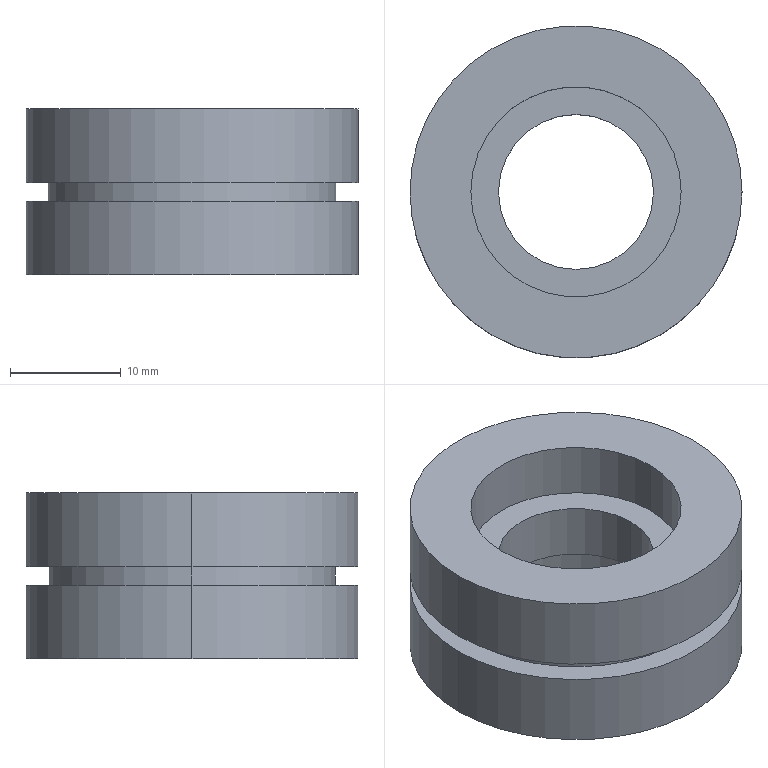Part | STEP file | 11-FG-B04111 | 1 solid | 18 faces | box 30 x 30 x 15 mm | volume 6699 mm3 | cylinder 12 | plane 6 | commonest cylinder face diameters 19 x4 30 x4 14 x2 26 x2
STEP:
#1=CARTESIAN_POINT('',(-13.,0.,8.35));
#2=VERTEX_POINT('',#1);
#3=CARTESIAN_POINT('',(13.,0.,8.35));
#4=VERTEX_POINT('',#3);
#5=CARTESIAN_POINT('',(0.,0.,8.35));
#6=DIRECTION('',(0.,0.,-1.));
#7=DIRECTION('',(-1.,0.,0.));
#8=AXIS2_PLACEMENT_3D('',#5,#6,#7);
#9=CIRCLE('',#8,13.);
#10=EDGE_CURVE('',#2,#4,#9,.T.);
#11=ORIENTED_EDGE('',*,*,#10,.T.);
#12=CARTESIAN_POINT('',(13.,0.,6.65));
#13=VERTEX_POINT('',#12);
#14=CARTESIAN_POINT('',(13.,0.,8.35));
#15=DIRECTION('',(0.,0.,-1.));
#16=VECTOR('',#15,1000.);
#17=LINE('',#14,#16);
#18=EDGE_CURVE('',#4,#13,#17,.T.);
#19=ORIENTED_EDGE('',*,*,#18,.T.);
#20=CARTESIAN_POINT('',(-13.,0.,6.65));
#21=VERTEX_POINT('',#20);
#22=CARTESIAN_POINT('',(0.,0.,6.65));
#23=DIRECTION('',(0.,0.,-1.));
#24=DIRECTION('',(-1.,0.,0.));
#25=AXIS2_PLACEMENT_3D('',#22,#23,#24);
#26=CIRCLE('',#25,13.);
#27=EDGE_CURVE('',#21,#13,#26,.T.);
#28=ORIENTED_EDGE('',*,*,#27,.F.);
#29=CARTESIAN_POINT('',(-13.,0.,8.35));
#30=DIRECTION('',(0.,0.,-1.));
#31=VECTOR('',#30,1000.);
#32=LINE('',#29,#31);
#33=EDGE_CURVE('',#2,#21,#32,.T.);
#34=ORIENTED_EDGE('',*,*,#33,.F.);
#35=EDGE_LOOP('',(#11,#19,#28,#34));
#36=FACE_OUTER_BOUND('',#35,.T.);
#37=CARTESIAN_POINT('',(0.,0.,8.35));
#38=DIRECTION('',(0.,0.,-1.));
#39=DIRECTION('',(-1.,0.,0.));
#40=AXIS2_PLACEMENT_3D('',#37,#38,#39);
#41=CYLINDRICAL_SURFACE('',#40,13.);
#42=ADVANCED_FACE('',(#36),#41,.T.);
#43=CARTESIAN_POINT('',(-9.5,0.,10.));
#44=VERTEX_POINT('',#43);
#45=CARTESIAN_POINT('',(9.5,0.,10.));
#46=VERTEX_POINT('',#45);
#47=CARTESIAN_POINT('',(0.,0.,10.));
#48=DIRECTION('',(0.,0.,1.));
#49=DIRECTION('',(1.,0.,0.));
#50=AXIS2_PLACEMENT_3D('',#47,#48,#49);
#51=CIRCLE('',#50,9.5);
#52=EDGE_CURVE('',#44,#46,#51,.T.);
#53=ORIENTED_EDGE('',*,*,#52,.F.);
#54=CARTESIAN_POINT('',(-9.5,0.,15.));
#55=VERTEX_POINT('',#54);
#56=CARTESIAN_POINT('',(-9.5,0.,10.));
#57=DIRECTION('',(0.,0.,1.));
#58=VECTOR('',#57,1000.);
#59=LINE('',#56,#58);
#60=EDGE_CURVE('',#44,#55,#59,.T.);
#61=ORIENTED_EDGE('',*,*,#60,.T.);
#62=CARTESIAN_POINT('',(9.5,0.,15.));
#63=VERTEX_POINT('',#62);
#64=CARTESIAN_POINT('',(0.,0.,15.));
#65=DIRECTION('',(0.,0.,1.));
#66=DIRECTION('',(1.,0.,0.));
#67=AXIS2_PLACEMENT_3D('',#64,#65,#66);
#68=CIRCLE('',#67,9.5);
#69=EDGE_CURVE('',#55,#63,#68,.T.);
#70=ORIENTED_EDGE('',*,*,#69,.T.);
#71=CARTESIAN_POINT('',(9.5,0.,10.));
#72=DIRECTION('',(0.,0.,1.));
#73=VECTOR('',#72,1000.);
#74=LINE('',#71,#73);
#75=EDGE_CURVE('',#46,#63,#74,.T.);
#76=ORIENTED_EDGE('',*,*,#75,.F.);
#77=EDGE_LOOP('',(#53,#61,#70,#76));
#78=FACE_OUTER_BOUND('',#77,.T.);
#79=CARTESIAN_POINT('',(0.,0.,10.));
#80=DIRECTION('',(0.,0.,1.));
#81=DIRECTION('',(1.,0.,0.));
#82=AXIS2_PLACEMENT_3D('',#79,#80,#81);
#83=CYLINDRICAL_SURFACE('',#82,9.5);
#84=ADVANCED_FACE('',(#78),#83,.F.);
#85=CARTESIAN_POINT('',(9.5,0.,5.));
#86=VERTEX_POINT('',#85);
#87=CARTESIAN_POINT('',(-9.5,0.,5.));
#88=VERTEX_POINT('',#87);
#89=CARTESIAN_POINT('',(0.,0.,5.));
#90=DIRECTION('',(0.,0.,-1.));
#91=DIRECTION('',(-1.,0.,0.));
#92=AXIS2_PLACEMENT_3D('',#89,#90,#91);
#93=CIRCLE('',#92,9.5);
#94=EDGE_CURVE('',#86,#88,#93,.T.);
#95=ORIENTED_EDGE('',*,*,#94,.F.);
#96=CARTESIAN_POINT('',(9.5,0.,0.));
#97=VERTEX_POINT('',#96);
#98=CARTESIAN_POINT('',(9.5,0.,5.));
#99=DIRECTION('',(0.,0.,-1.));
#100=VECTOR('',#99,1000.);
#101=LINE('',#98,#100);
#102=EDGE_CURVE('',#86,#97,#101,.T.);
#103=ORIENTED_EDGE('',*,*,#102,.T.);
#104=CARTESIAN_POINT('',(-9.5,0.,0.));
#105=VERTEX_POINT('',#104);
#106=CARTESIAN_POINT('',(0.,0.,0.));
#107=DIRECTION('',(0.,0.,-1.));
#108=DIRECTION('',(-1.,0.,0.));
#109=AXIS2_PLACEMENT_3D('',#106,#107,#108);
#110=CIRCLE('',#109,9.5);
#111=EDGE_CURVE('',#97,#105,#110,.T.);
#112=ORIENTED_EDGE('',*,*,#111,.T.);
#113=CARTESIAN_POINT('',(-9.5,0.,5.));
#114=DIRECTION('',(0.,0.,-1.));
#115=VECTOR('',#114,1000.);
#116=LINE('',#113,#115);
#117=EDGE_CURVE('',#88,#105,#116,.T.);
#118=ORIENTED_EDGE('',*,*,#117,.F.);
#119=EDGE_LOOP('',(#95,#103,#112,#118));
#120=FACE_OUTER_BOUND('',#119,.T.);
#121=CARTESIAN_POINT('',(0.,0.,5.));
#122=DIRECTION('',(0.,0.,-1.));
#123=DIRECTION('',(-1.,0.,0.));
#124=AXIS2_PLACEMENT_3D('',#121,#122,#123);
#125=CYLINDRICAL_SURFACE('',#124,9.5);
#126=ADVANCED_FACE('',(#120),#125,.F.);
#127=CARTESIAN_POINT('',(-15.,0.,6.65));
#128=VERTEX_POINT('',#127);
#129=CARTESIAN_POINT('',(15.,0.,6.65));
#130=VERTEX_POINT('',#129);
#131=CARTESIAN_POINT('',(0.,0.,6.65));
#132=DIRECTION('',(0.,0.,-1.));
#133=DIRECTION('',(-1.,0.,0.));
#134=AXIS2_PLACEMENT_3D('',#131,#132,#133);
#135=CIRCLE('',#134,15.);
#136=EDGE_CURVE('',#128,#130,#135,.T.);
#137=ORIENTED_EDGE('',*,*,#136,.T.);
#138=CARTESIAN_POINT('',(15.,0.,0.));
#139=VERTEX_POINT('',#138);
#140=CARTESIAN_POINT('',(15.,0.,15.));
#141=DIRECTION('',(0.,0.,-1.));
#142=VECTOR('',#141,1000.);
#143=LINE('',#140,#142);
#144=EDGE_CURVE('',#130,#139,#143,.T.);
#145=ORIENTED_EDGE('',*,*,#144,.T.);
#146=CARTESIAN_POINT('',(-15.,0.,0.));
#147=VERTEX_POINT('',#146);
#148=CARTESIAN_POINT('',(0.,0.,0.));
#149=DIRECTION('',(0.,0.,1.));
#150=DIRECTION('',(1.,0.,0.));
#151=AXIS2_PLACEMENT_3D('',#148,#149,#150);
#152=CIRCLE('',#151,15.);
#153=EDGE_CURVE('',#139,#147,#152,.T.);
#154=ORIENTED_EDGE('',*,*,#153,.T.);
#155=CARTESIAN_POINT('',(-15.,0.,15.));
#156=DIRECTION('',(0.,0.,-1.));
#157=VECTOR('',#156,1000.);
#158=LINE('',#155,#157);
#159=EDGE_CURVE('',#128,#147,#158,.T.);
#160=ORIENTED_EDGE('',*,*,#159,.F.);
#161=EDGE_LOOP('',(#137,#145,#154,#160));
#162=FACE_OUTER_BOUND('',#161,.T.);
#163=CARTESIAN_POINT('',(0.,0.,15.));
#164=DIRECTION('',(0.,0.,-1.));
#165=DIRECTION('',(-1.,0.,0.));
#166=AXIS2_PLACEMENT_3D('',#163,#164,#165);
#167=CYLINDRICAL_SURFACE('',#166,15.);
#168=ADVANCED_FACE('',(#162),#167,.T.);
#169=CARTESIAN_POINT('',(7.,0.,10.));
#170=VERTEX_POINT('',#169);
#171=CARTESIAN_POINT('',(-7.,0.,10.));
#172=VERTEX_POINT('',#171);
#173=CARTESIAN_POINT('',(0.,0.,10.));
#174=DIRECTION('',(0.,0.,-1.));
#175=DIRECTION('',(1.,0.,0.));
#176=AXIS2_PLACEMENT_3D('',#173,#174,#175);
#177=CIRCLE('',#176,7.);
#178=EDGE_CURVE('',#170,#172,#177,.T.);
#179=ORIENTED_EDGE('',*,*,#178,.F.);
#180=CARTESIAN_POINT('',(7.,0.,5.));
#181=VERTEX_POINT('',#180);
#182=CARTESIAN_POINT('',(7.,0.,26.));
#183=DIRECTION('',(0.,0.,-1.));
#184=VECTOR('',#183,1000.);
#185=LINE('',#182,#184);
#186=EDGE_CURVE('',#170,#181,#185,.T.);
#187=ORIENTED_EDGE('',*,*,#186,.T.);
#188=CARTESIAN_POINT('',(-7.,0.,5.));
#189=VERTEX_POINT('',#188);
#190=CARTESIAN_POINT('',(0.,0.,5.));
#191=DIRECTION('',(0.,0.,1.));
#192=DIRECTION('',(-1.,0.,0.));
#193=AXIS2_PLACEMENT_3D('',#190,#191,#192);
#194=CIRCLE('',#193,7.);
#195=EDGE_CURVE('',#189,#181,#194,.T.);
#196=ORIENTED_EDGE('',*,*,#195,.F.);
#197=CARTESIAN_POINT('',(-7.,0.,26.));
#198=DIRECTION('',(0.,0.,-1.));
#199=VECTOR('',#198,1000.);
#200=LINE('',#197,#199);
#201=EDGE_CURVE('',#172,#189,#200,.T.);
#202=ORIENTED_EDGE('',*,*,#201,.F.);
#203=EDGE_LOOP('',(#179,#187,#196,#202));
#204=FACE_OUTER_BOUND('',#203,.T.);
#205=CARTESIAN_POINT('',(0.,0.,26.));
#206=DIRECTION('',(0.,0.,-1.));
#207=DIRECTION('',(-1.,0.,0.));
#208=AXIS2_PLACEMENT_3D('',#205,#206,#207);
#209=CYLINDRICAL_SURFACE('',#208,7.);
#210=ADVANCED_FACE('',(#204),#209,.F.);
#211=CARTESIAN_POINT('',(15.,0.,15.));
#212=VERTEX_POINT('',#211);
#213=CARTESIAN_POINT('',(-15.,0.,15.));
#214=VERTEX_POINT('',#213);
#215=CARTESIAN_POINT('',(0.,0.,15.));
#216=DIRECTION('',(0.,0.,1.));
#217=DIRECTION('',(1.,0.,0.));
#218=AXIS2_PLACEMENT_3D('',#215,#216,#217);
#219=CIRCLE('',#218,15.);
#220=EDGE_CURVE('',#212,#214,#219,.T.);
#221=ORIENTED_EDGE('',*,*,#220,.F.);
#222=CARTESIAN_POINT('',(15.,0.,8.35));
#223=VERTEX_POINT('',#222);
#224=CARTESIAN_POINT('',(15.,0.,15.));
#225=DIRECTION('',(0.,0.,-1.));
#226=VECTOR('',#225,1000.);
#227=LINE('',#224,#226);
#228=EDGE_CURVE('',#212,#223,#227,.T.);
#229=ORIENTED_EDGE('',*,*,#228,.T.);
#230=CARTESIAN_POINT('',(-15.,0.,8.35));
#231=VERTEX_POINT('',#230);
#232=CARTESIAN_POINT('',(0.,0.,8.35));
#233=DIRECTION('',(0.,0.,-1.));
#234=DIRECTION('',(-1.,0.,0.));
#235=AXIS2_PLACEMENT_3D('',#232,#233,#234);
#236=CIRCLE('',#235,15.);
#237=EDGE_CURVE('',#231,#223,#236,.T.);
#238=ORIENTED_EDGE('',*,*,#237,.F.);
#239=CARTESIAN_POINT('',(-15.,0.,15.));
#240=DIRECTION('',(0.,0.,-1.));
#241=VECTOR('',#240,1000.);
#242=LINE('',#239,#241);
#243=EDGE_CURVE('',#214,#231,#242,.T.);
#244=ORIENTED_EDGE('',*,*,#243,.F.);
#245=EDGE_LOOP('',(#221,#229,#238,#244));
#246=FACE_OUTER_BOUND('',#245,.T.);
#247=CARTESIAN_POINT('',(0.,0.,15.));
#248=DIRECTION('',(0.,0.,-1.));
#249=DIRECTION('',(-1.,0.,0.));
#250=AXIS2_PLACEMENT_3D('',#247,#248,#249);
#251=CYLINDRICAL_SURFACE('',#250,15.);
#252=ADVANCED_FACE('',(#246),#251,.T.);
#253=ORIENTED_EDGE('',*,*,#228,.F.);
#254=CARTESIAN_POINT('',(0.,0.,15.));
#255=DIRECTION('',(0.,0.,1.));
#256=DIRECTION('',(1.,0.,0.));
#257=AXIS2_PLACEMENT_3D('',#254,#255,#256);
#258=CIRCLE('',#257,15.);
#259=EDGE_CURVE('',#214,#212,#258,.T.);
#260=ORIENTED_EDGE('',*,*,#259,.F.);
#261=ORIENTED_EDGE('',*,*,#243,.T.);
#262=CARTESIAN_POINT('',(0.,0.,8.35));
#263=DIRECTION('',(0.,0.,-1.));
#264=DIRECTION('',(-1.,0.,0.));
#265=AXIS2_PLACEMENT_3D('',#262,#263,#264);
#266=CIRCLE('',#265,15.);
#267=EDGE_CURVE('',#223,#231,#266,.T.);
#268=ORIENTED_EDGE('',*,*,#267,.F.);
#269=EDGE_LOOP('',(#253,#260,#261,#268));
#270=FACE_OUTER_BOUND('',#269,.T.);
#271=CARTESIAN_POINT('',(0.,0.,15.));
#272=DIRECTION('',(0.,0.,-1.));
#273=DIRECTION('',(-1.,0.,0.));
#274=AXIS2_PLACEMENT_3D('',#271,#272,#273);
#275=CYLINDRICAL_SURFACE('',#274,15.);
#276=ADVANCED_FACE('',(#270),#275,.T.);
#277=ORIENTED_EDGE('',*,*,#186,.F.);
#278=CARTESIAN_POINT('',(0.,0.,10.));
#279=DIRECTION('',(0.,0.,-1.));
#280=DIRECTION('',(1.,0.,0.));
#281=AXIS2_PLACEMENT_3D('',#278,#279,#280);
#282=CIRCLE('',#281,7.);
#283=EDGE_CURVE('',#172,#170,#282,.T.);
#284=ORIENTED_EDGE('',*,*,#283,.F.);
#285=ORIENTED_EDGE('',*,*,#201,.T.);
#286=CARTESIAN_POINT('',(0.,0.,5.));
#287=DIRECTION('',(0.,0.,1.));
#288=DIRECTION('',(-1.,0.,0.));
#289=AXIS2_PLACEMENT_3D('',#286,#287,#288);
#290=CIRCLE('',#289,7.);
#291=EDGE_CURVE('',#181,#189,#290,.T.);
#292=ORIENTED_EDGE('',*,*,#291,.F.);
#293=EDGE_LOOP('',(#277,#284,#285,#292));
#294=FACE_OUTER_BOUND('',#293,.T.);
#295=CARTESIAN_POINT('',(0.,0.,26.));
#296=DIRECTION('',(0.,0.,-1.));
#297=DIRECTION('',(-1.,0.,0.));
#298=AXIS2_PLACEMENT_3D('',#295,#296,#297);
#299=CYLINDRICAL_SURFACE('',#298,7.);
#300=ADVANCED_FACE('',(#294),#299,.F.);
#301=ORIENTED_EDGE('',*,*,#144,.F.);
#302=CARTESIAN_POINT('',(0.,0.,6.65));
#303=DIRECTION('',(0.,0.,-1.));
#304=DIRECTION('',(-1.,0.,0.));
#305=AXIS2_PLACEMENT_3D('',#302,#303,#304);
#306=CIRCLE('',#305,15.);
#307=EDGE_CURVE('',#130,#128,#306,.T.);
#308=ORIENTED_EDGE('',*,*,#307,.T.);
#309=ORIENTED_EDGE('',*,*,#159,.T.);
#310=CARTESIAN_POINT('',(0.,0.,0.));
#311=DIRECTION('',(0.,0.,1.));
#312=DIRECTION('',(1.,0.,0.));
#313=AXIS2_PLACEMENT_3D('',#310,#311,#312);
#314=CIRCLE('',#313,15.);
#315=EDGE_CURVE('',#147,#139,#314,.T.);
#316=ORIENTED_EDGE('',*,*,#315,.T.);
#317=EDGE_LOOP('',(#301,#308,#309,#316));
#318=FACE_OUTER_BOUND('',#317,.T.);
#319=CARTESIAN_POINT('',(0.,0.,15.));
#320=DIRECTION('',(0.,0.,-1.));
#321=DIRECTION('',(-1.,0.,0.));
#322=AXIS2_PLACEMENT_3D('',#319,#320,#321);
#323=CYLINDRICAL_SURFACE('',#322,15.);
#324=ADVANCED_FACE('',(#318),#323,.T.);
#325=CARTESIAN_POINT('',(0.,0.,15.));
#326=DIRECTION('',(0.,0.,1.));
#327=DIRECTION('',(1.,0.,0.));
#328=AXIS2_PLACEMENT_3D('',#325,#326,#327);
#329=CIRCLE('',#328,9.5);
#330=EDGE_CURVE('',#63,#55,#329,.T.);
#331=ORIENTED_EDGE('',*,*,#330,.F.);
#332=ORIENTED_EDGE('',*,*,#69,.F.);
#333=EDGE_LOOP('',(#331,#332));
#334=FACE_BOUND('',#333,.T.);
#335=ORIENTED_EDGE('',*,*,#259,.T.);
#336=ORIENTED_EDGE('',*,*,#220,.T.);
#337=EDGE_LOOP('',(#335,#336));
#338=FACE_OUTER_BOUND('',#337,.T.);
#339=CARTESIAN_POINT('',(0.,0.,15.));
#340=DIRECTION('',(0.,0.,1.));
#341=DIRECTION('',(1.,0.,0.));
#342=AXIS2_PLACEMENT_3D('',#339,#340,#341);
#343=PLANE('',#342);
#344=ADVANCED_FACE('',(#334,#338),#343,.T.);
#345=CARTESIAN_POINT('',(0.,0.,0.));
#346=DIRECTION('',(0.,0.,-1.));
#347=DIRECTION('',(-1.,0.,0.));
#348=AXIS2_PLACEMENT_3D('',#345,#346,#347);
#349=CIRCLE('',#348,9.5);
#350=EDGE_CURVE('',#105,#97,#349,.T.);
#351=ORIENTED_EDGE('',*,*,#350,.F.);
#352=ORIENTED_EDGE('',*,*,#111,.F.);
#353=EDGE_LOOP('',(#351,#352));
#354=FACE_BOUND('',#353,.T.);
#355=ORIENTED_EDGE('',*,*,#315,.F.);
#356=ORIENTED_EDGE('',*,*,#153,.F.);
#357=EDGE_LOOP('',(#355,#356));
#358=FACE_OUTER_BOUND('',#357,.T.);
#359=CARTESIAN_POINT('',(0.,0.,0.));
#360=DIRECTION('',(0.,0.,1.));
#361=DIRECTION('',(1.,0.,0.));
#362=AXIS2_PLACEMENT_3D('',#359,#360,#361);
#363=PLANE('',#362);
#364=ADVANCED_FACE('',(#354,#358),#363,.F.);
#365=CARTESIAN_POINT('',(0.,0.,5.));
#366=DIRECTION('',(0.,0.,-1.));
#367=DIRECTION('',(-1.,0.,0.));
#368=AXIS2_PLACEMENT_3D('',#365,#366,#367);
#369=CIRCLE('',#368,9.5);
#370=EDGE_CURVE('',#88,#86,#369,.T.);
#371=ORIENTED_EDGE('',*,*,#370,.T.);
#372=ORIENTED_EDGE('',*,*,#94,.T.);
#373=EDGE_LOOP('',(#371,#372));
#374=FACE_OUTER_BOUND('',#373,.T.);
#375=ORIENTED_EDGE('',*,*,#195,.T.);
#376=ORIENTED_EDGE('',*,*,#291,.T.);
#377=EDGE_LOOP('',(#375,#376));
#378=FACE_BOUND('',#377,.T.);
#379=CARTESIAN_POINT('',(0.,0.,5.));
#380=DIRECTION('',(0.,0.,-1.));
#381=DIRECTION('',(-1.,0.,0.));
#382=AXIS2_PLACEMENT_3D('',#379,#380,#381);
#383=PLANE('',#382);
#384=ADVANCED_FACE('',(#374,#378),#383,.T.);
#385=ORIENTED_EDGE('',*,*,#102,.F.);
#386=ORIENTED_EDGE('',*,*,#370,.F.);
#387=ORIENTED_EDGE('',*,*,#117,.T.);
#388=ORIENTED_EDGE('',*,*,#350,.T.);
#389=EDGE_LOOP('',(#385,#386,#387,#388));
#390=FACE_OUTER_BOUND('',#389,.T.);
#391=CARTESIAN_POINT('',(0.,0.,5.));
#392=DIRECTION('',(0.,0.,-1.));
#393=DIRECTION('',(-1.,0.,0.));
#394=AXIS2_PLACEMENT_3D('',#391,#392,#393);
#395=CYLINDRICAL_SURFACE('',#394,9.5);
#396=ADVANCED_FACE('',(#390),#395,.F.);
#397=CARTESIAN_POINT('',(0.,0.,10.));
#398=DIRECTION('',(0.,0.,1.));
#399=DIRECTION('',(1.,0.,0.));
#400=AXIS2_PLACEMENT_3D('',#397,#398,#399);
#401=CIRCLE('',#400,9.5);
#402=EDGE_CURVE('',#46,#44,#401,.T.);
#403=ORIENTED_EDGE('',*,*,#402,.T.);
#404=ORIENTED_EDGE('',*,*,#52,.T.);
#405=EDGE_LOOP('',(#403,#404));
#406=FACE_OUTER_BOUND('',#405,.T.);
#407=ORIENTED_EDGE('',*,*,#283,.T.);
#408=ORIENTED_EDGE('',*,*,#178,.T.);
#409=EDGE_LOOP('',(#407,#408));
#410=FACE_BOUND('',#409,.T.);
#411=CARTESIAN_POINT('',(0.,0.,10.));
#412=DIRECTION('',(0.,0.,1.));
#413=DIRECTION('',(1.,0.,0.));
#414=AXIS2_PLACEMENT_3D('',#411,#412,#413);
#415=PLANE('',#414);
#416=ADVANCED_FACE('',(#406,#410),#415,.T.);
#417=ORIENTED_EDGE('',*,*,#60,.F.);
#418=ORIENTED_EDGE('',*,*,#402,.F.);
#419=ORIENTED_EDGE('',*,*,#75,.T.);
#420=ORIENTED_EDGE('',*,*,#330,.T.);
#421=EDGE_LOOP('',(#417,#418,#419,#420));
#422=FACE_OUTER_BOUND('',#421,.T.);
#423=CARTESIAN_POINT('',(0.,0.,10.));
#424=DIRECTION('',(0.,0.,1.));
#425=DIRECTION('',(1.,0.,0.));
#426=AXIS2_PLACEMENT_3D('',#423,#424,#425);
#427=CYLINDRICAL_SURFACE('',#426,9.5);
#428=ADVANCED_FACE('',(#422),#427,.F.);
#429=ORIENTED_EDGE('',*,*,#10,.F.);
#430=CARTESIAN_POINT('',(0.,0.,8.35));
#431=DIRECTION('',(0.,0.,-1.));
#432=DIRECTION('',(-1.,0.,0.));
#433=AXIS2_PLACEMENT_3D('',#430,#431,#432);
#434=CIRCLE('',#433,13.);
#435=EDGE_CURVE('',#4,#2,#434,.T.);
#436=ORIENTED_EDGE('',*,*,#435,.F.);
#437=EDGE_LOOP('',(#429,#436));
#438=FACE_BOUND('',#437,.T.);
#439=ORIENTED_EDGE('',*,*,#237,.T.);
#440=ORIENTED_EDGE('',*,*,#267,.T.);
#441=EDGE_LOOP('',(#439,#440));
#442=FACE_OUTER_BOUND('',#441,.T.);
#443=CARTESIAN_POINT('',(0.,0.,8.35));
#444=DIRECTION('',(0.,0.,-1.));
#445=DIRECTION('',(-1.,0.,0.));
#446=AXIS2_PLACEMENT_3D('',#443,#444,#445);
#447=PLANE('',#446);
#448=ADVANCED_FACE('',(#438,#442),#447,.T.);
#449=ORIENTED_EDGE('',*,*,#27,.T.);
#450=CARTESIAN_POINT('',(0.,0.,6.65));
#451=DIRECTION('',(0.,0.,-1.));
#452=DIRECTION('',(-1.,0.,0.));
#453=AXIS2_PLACEMENT_3D('',#450,#451,#452);
#454=CIRCLE('',#453,13.);
#455=EDGE_CURVE('',#13,#21,#454,.T.);
#456=ORIENTED_EDGE('',*,*,#455,.T.);
#457=EDGE_LOOP('',(#449,#456));
#458=FACE_BOUND('',#457,.T.);
#459=ORIENTED_EDGE('',*,*,#136,.F.);
#460=ORIENTED_EDGE('',*,*,#307,.F.);
#461=EDGE_LOOP('',(#459,#460));
#462=FACE_OUTER_BOUND('',#461,.T.);
#463=CARTESIAN_POINT('',(0.,0.,6.65));
#464=DIRECTION('',(0.,0.,-1.));
#465=DIRECTION('',(-1.,0.,0.));
#466=AXIS2_PLACEMENT_3D('',#463,#464,#465);
#467=PLANE('',#466);
#468=ADVANCED_FACE('',(#458,#462),#467,.F.);
#469=ORIENTED_EDGE('',*,*,#18,.F.);
#470=ORIENTED_EDGE('',*,*,#435,.T.);
#471=ORIENTED_EDGE('',*,*,#33,.T.);
#472=ORIENTED_EDGE('',*,*,#455,.F.);
#473=EDGE_LOOP('',(#469,#470,#471,#472));
#474=FACE_OUTER_BOUND('',#473,.T.);
#475=CARTESIAN_POINT('',(0.,0.,8.35));
#476=DIRECTION('',(0.,0.,-1.));
#477=DIRECTION('',(-1.,0.,0.));
#478=AXIS2_PLACEMENT_3D('',#475,#476,#477);
#479=CYLINDRICAL_SURFACE('',#478,13.);
#480=ADVANCED_FACE('',(#474),#479,.T.);
#481=CLOSED_SHELL('',(#42,#84,#126,#168,#210,#252,#276,#300,#324,#344,#364,#384,#396,#416,#428,#448,#468,#480));
#482=MANIFOLD_SOLID_BREP('',#481);
#483=CARTESIAN_POINT('',(0.,0.,0.));
#484=DIRECTION('',(0.,0.,1.));
#485=DIRECTION('',(1.,0.,0.));
#486=AXIS2_PLACEMENT_3D('',#483,#484,#485);
#487=(LENGTH_UNIT()NAMED_UNIT(*)SI_UNIT(.MILLI.,.METRE.));
#488=UNCERTAINTY_MEASURE_WITH_UNIT(LENGTH_MEASURE(0.00001),#487,'','');
#489=(NAMED_UNIT(*)PLANE_ANGLE_UNIT()SI_UNIT($,.RADIAN.));
#490=(NAMED_UNIT(*)SI_UNIT($,.STERADIAN.)SOLID_ANGLE_UNIT());
#491=(GEOMETRIC_REPRESENTATION_CONTEXT(3)GLOBAL_UNCERTAINTY_ASSIGNED_CONTEXT((#488))GLOBAL_UNIT_ASSIGNED_CONTEXT((#487,#489,#490))REPRESENTATION_CONTEXT('',''));
#492=ADVANCED_BREP_SHAPE_REPRESENTATION('',(#482,#486),#491);